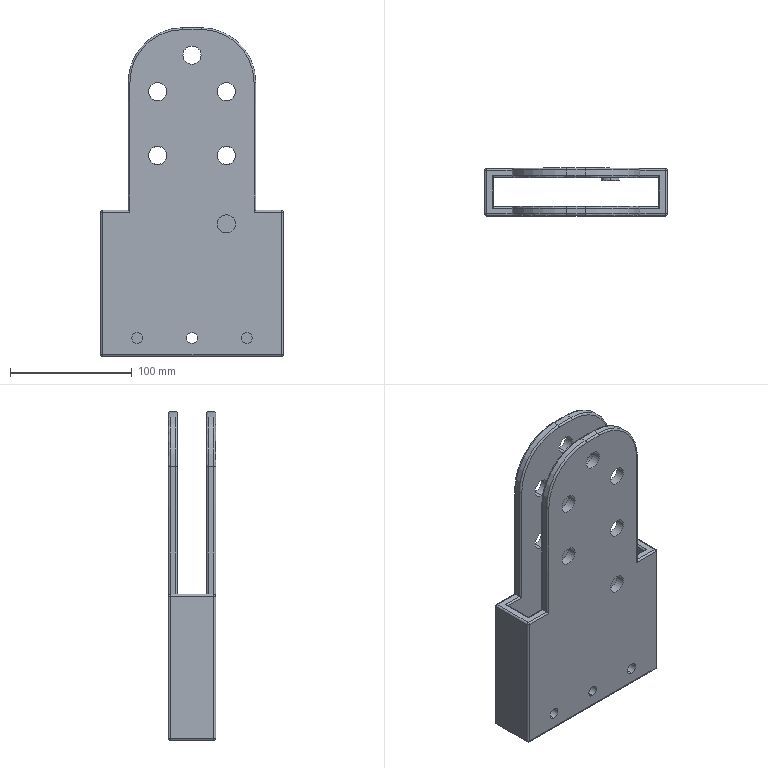Part | SolidWorks | features ICE 2, 3DProfileFeature 1, BaseBody 1, HoleWzd 1 | 2 solids | 126 faces | box 150 x 39 x 270 mm | volume 515829 mm3 | cylinder 90 | plane 20 | spline 16 | commonest cylinder face diameters 3 x36 15 x30 9 x12 5 x8 90 x4